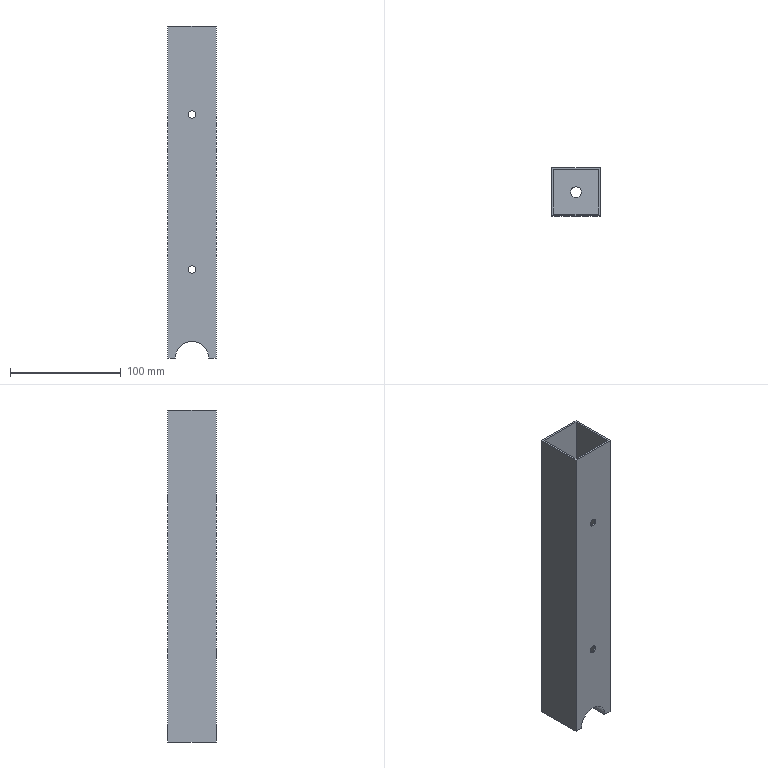Part | SolidWorks | features ICE 3, Extrusion 1, HoleWzd 1 | 1 solid | 28 faces | box 43.5 x 43.5 x 300 mm | volume 108012 mm3 | cylinder 12 | plane 12 | cone 4 | commonest cylinder face diameters 6.8 x8 10 x2 30 x2
STEP:
#1=CARTESIAN_POINT('',(-15.25,20.25,30.));
#2=VERTEX_POINT('',#1);
#3=CARTESIAN_POINT('',(-25.25,20.25,30.));
#4=VERTEX_POINT('',#3);
#5=CARTESIAN_POINT('',(-20.25,20.25,30.));
#6=DIRECTION('',(0.,0.,-1.));
#7=DIRECTION('',(-1.,0.,0.));
#8=AXIS2_PLACEMENT_3D('',#5,#6,#7);
#9=CIRCLE('',#8,5.);
#10=EDGE_CURVE('',#2,#4,#9,.T.);
#11=ORIENTED_EDGE('',*,*,#10,.F.);
#12=CARTESIAN_POINT('',(-15.25,20.25,14.142));
#13=VERTEX_POINT('',#12);
#14=CARTESIAN_POINT('',(-15.25,20.25,300.));
#15=DIRECTION('',(0.,0.,-1.));
#16=VECTOR('',#15,1000.);
#17=LINE('',#14,#16);
#18=EDGE_CURVE('',#2,#13,#17,.T.);
#19=ORIENTED_EDGE('',*,*,#18,.T.);
#20=CARTESIAN_POINT('',(-20.25,15.25,15.));
#21=VERTEX_POINT('',#20);
#22=CARTESIAN_POINT('',(-20.25,15.25,15.));
#23=CARTESIAN_POINT('',(-19.921,15.25,15.));
#24=CARTESIAN_POINT('',(-19.587,15.283,14.989));
#25=CARTESIAN_POINT('',(-18.944,15.412,14.947));
#26=CARTESIAN_POINT('',(-18.631,15.508,14.916));
#27=CARTESIAN_POINT('',(-18.023,15.761,14.837));
#28=CARTESIAN_POINT('',(-17.735,15.917,14.79));
#29=CARTESIAN_POINT('',(-17.196,16.278,14.688));
#30=CARTESIAN_POINT('',(-16.941,16.487,14.632));
#31=CARTESIAN_POINT('',(-16.481,16.948,14.521));
#32=CARTESIAN_POINT('',(-16.276,17.198,14.465));
#33=CARTESIAN_POINT('',(-15.915,17.738,14.361));
#34=CARTESIAN_POINT('',(-15.758,18.03,14.312));
#35=CARTESIAN_POINT('',(-15.508,18.632,14.231));
#36=CARTESIAN_POINT('',(-15.412,18.944,14.199));
#37=CARTESIAN_POINT('',(-15.315,19.429,14.165));
#38=CARTESIAN_POINT('',(-15.29,19.594,14.156));
#39=CARTESIAN_POINT('',(-15.258,19.922,14.145));
#40=CARTESIAN_POINT('',(-15.25,20.086,14.142));
#41=CARTESIAN_POINT('',(-15.25,20.25,14.142));
#42=B_SPLINE_CURVE_WITH_KNOTS('',3,(#22,#23,#24,#25,#26,#27,#28,#29,#30,#31,#32,#33,#34,#35,#36,#37,#38,#39,#40,#41),.UNSPECIFIED.,.F.,.F.,(4,2,2,2,2,2,2,2,2,4),(0.007875,0.008859,0.009843,0.01083,0.01181,0.01279,0.01378,0.01476,0.01525,0.01575),.UNSPECIFIED.);
#43=EDGE_CURVE('',#21,#13,#42,.T.);
#44=ORIENTED_EDGE('',*,*,#43,.F.);
#45=CARTESIAN_POINT('',(-25.25,20.25,14.142));
#46=VERTEX_POINT('',#45);
#47=CARTESIAN_POINT('',(-25.25,20.25,14.142));
#48=CARTESIAN_POINT('',(-25.25,19.917,14.142));
#49=CARTESIAN_POINT('',(-25.217,19.59,14.154));
#50=CARTESIAN_POINT('',(-25.088,18.948,14.198));
#51=CARTESIAN_POINT('',(-24.991,18.629,14.232));
#52=CARTESIAN_POINT('',(-24.739,18.024,14.313));
#53=CARTESIAN_POINT('',(-24.585,17.738,14.361));
#54=CARTESIAN_POINT('',(-24.223,17.196,14.466));
#55=CARTESIAN_POINT('',(-24.013,16.942,14.522));
#56=CARTESIAN_POINT('',(-23.555,16.484,14.633));
#57=CARTESIAN_POINT('',(-23.305,16.278,14.688));
#58=CARTESIAN_POINT('',(-22.758,15.912,14.791));
#59=CARTESIAN_POINT('',(-22.471,15.759,14.838));
#60=CARTESIAN_POINT('',(-22.02,15.571,14.896));
#61=CARTESIAN_POINT('',(-21.867,15.516,14.913));
#62=CARTESIAN_POINT('',(-21.552,15.42,14.944));
#63=CARTESIAN_POINT('',(-21.39,15.379,14.957));
#64=CARTESIAN_POINT('',(-20.905,15.282,14.989));
#65=CARTESIAN_POINT('',(-20.579,15.25,15.));
#66=CARTESIAN_POINT('',(-20.25,15.25,15.));
#67=B_SPLINE_CURVE_WITH_KNOTS('',3,(#47,#48,#49,#50,#51,#52,#53,#54,#55,#56,#57,#58,#59,#60,#61,#62,#63,#64,#65,#66),.UNSPECIFIED.,.F.,.F.,(4,2,2,2,2,2,2,2,2,4),(0.,0.0009844,0.001969,0.002953,0.003937,0.004922,0.005906,0.006398,0.006891,0.007875),.UNSPECIFIED.);
#68=EDGE_CURVE('',#46,#21,#67,.T.);
#69=ORIENTED_EDGE('',*,*,#68,.F.);
#70=CARTESIAN_POINT('',(-25.25,20.25,300.));
#71=DIRECTION('',(0.,0.,-1.));
#72=VECTOR('',#71,1000.);
#73=LINE('',#70,#72);
#74=EDGE_CURVE('',#4,#46,#73,.T.);
#75=ORIENTED_EDGE('',*,*,#74,.F.);
#76=EDGE_LOOP('',(#11,#19,#44,#69,#75));
#77=FACE_OUTER_BOUND('',#76,.T.);
#78=CARTESIAN_POINT('',(-20.25,20.25,300.));
#79=DIRECTION('',(0.,0.,-1.));
#80=DIRECTION('',(-1.,0.,0.));
#81=AXIS2_PLACEMENT_3D('',#78,#79,#80);
#82=CYLINDRICAL_SURFACE('',#81,5.);
#83=ADVANCED_FACE('',(#77),#82,.F.);
#84=CARTESIAN_POINT('',(-20.25,-1.5,15.));
#85=VERTEX_POINT('',#84);
#86=CARTESIAN_POINT('',(-5.25,-1.5,0.));
#87=VERTEX_POINT('',#86);
#88=CARTESIAN_POINT('',(-20.25,-1.5,0.));
#89=DIRECTION('',(0.,1.,0.));
#90=DIRECTION('',(0.,0.,1.));
#91=AXIS2_PLACEMENT_3D('',#88,#89,#90);
#92=CIRCLE('',#91,15.);
#93=EDGE_CURVE('',#85,#87,#92,.T.);
#94=ORIENTED_EDGE('',*,*,#93,.F.);
#95=CARTESIAN_POINT('',(-20.25,-1.5,15.));
#96=DIRECTION('',(0.,1.,0.));
#97=VECTOR('',#96,1000.);
#98=LINE('',#95,#97);
#99=EDGE_CURVE('',#85,#21,#98,.T.);
#100=ORIENTED_EDGE('',*,*,#99,.T.);
#101=ORIENTED_EDGE('',*,*,#43,.T.);
#102=CARTESIAN_POINT('',(-20.25,25.25,15.));
#103=VERTEX_POINT('',#102);
#104=CARTESIAN_POINT('',(-15.25,20.25,14.142));
#105=CARTESIAN_POINT('',(-15.25,20.578,14.142));
#106=CARTESIAN_POINT('',(-15.282,20.908,14.154));
#107=CARTESIAN_POINT('',(-15.412,21.556,14.199));
#108=CARTESIAN_POINT('',(-15.508,21.869,14.231));
#109=CARTESIAN_POINT('',(-15.759,22.472,14.313));
#110=CARTESIAN_POINT('',(-15.916,22.764,14.361));
#111=CARTESIAN_POINT('',(-16.278,23.304,14.466));
#112=CARTESIAN_POINT('',(-16.483,23.554,14.521));
#113=CARTESIAN_POINT('',(-16.945,24.016,14.633));
#114=CARTESIAN_POINT('',(-17.198,24.224,14.689));
#115=CARTESIAN_POINT('',(-17.736,24.584,14.79));
#116=CARTESIAN_POINT('',(-18.025,24.74,14.837));
#117=CARTESIAN_POINT('',(-18.633,24.993,14.916));
#118=CARTESIAN_POINT('',(-18.945,25.088,14.947));
#119=CARTESIAN_POINT('',(-19.587,25.217,14.989));
#120=CARTESIAN_POINT('',(-19.921,25.25,15.));
#121=CARTESIAN_POINT('',(-20.25,25.25,15.));
#122=B_SPLINE_CURVE_WITH_KNOTS('',3,(#104,#105,#106,#107,#108,#109,#110,#111,#112,#113,#114,#115,#116,#117,#118,#119,#120,#121),.UNSPECIFIED.,.F.,.F.,(4,2,2,2,2,2,2,2,4),(0.01575,0.01673,0.01771,0.0187,0.01968,0.02066,0.02165,0.02263,0.02362),.UNSPECIFIED.);
#123=EDGE_CURVE('',#13,#103,#122,.T.);
#124=ORIENTED_EDGE('',*,*,#123,.T.);
#125=CARTESIAN_POINT('',(-20.25,42.,15.));
#126=VERTEX_POINT('',#125);
#127=CARTESIAN_POINT('',(-20.25,-1.5,15.));
#128=DIRECTION('',(0.,1.,0.));
#129=VECTOR('',#128,1000.);
#130=LINE('',#127,#129);
#131=EDGE_CURVE('',#103,#126,#130,.T.);
#132=ORIENTED_EDGE('',*,*,#131,.T.);
#133=CARTESIAN_POINT('',(-5.25,42.,0.));
#134=VERTEX_POINT('',#133);
#135=CARTESIAN_POINT('',(-20.25,42.,0.));
#136=DIRECTION('',(0.,1.,0.));
#137=DIRECTION('',(0.,0.,1.));
#138=AXIS2_PLACEMENT_3D('',#135,#136,#137);
#139=CIRCLE('',#138,15.);
#140=EDGE_CURVE('',#126,#134,#139,.T.);
#141=ORIENTED_EDGE('',*,*,#140,.T.);
#142=CARTESIAN_POINT('',(-5.25,-1.5,0.));
#143=DIRECTION('',(0.,1.,0.));
#144=VECTOR('',#143,1000.);
#145=LINE('',#142,#144);
#146=EDGE_CURVE('',#87,#134,#145,.T.);
#147=ORIENTED_EDGE('',*,*,#146,.F.);
#148=EDGE_LOOP('',(#94,#100,#101,#124,#132,#141,#147));
#149=FACE_OUTER_BOUND('',#148,.T.);
#150=CARTESIAN_POINT('',(-20.25,-1.5,0.));
#151=DIRECTION('',(0.,1.,0.));
#152=DIRECTION('',(0.,0.,1.));
#153=AXIS2_PLACEMENT_3D('',#150,#151,#152);
#154=CYLINDRICAL_SURFACE('',#153,15.);
#155=ADVANCED_FACE('',(#149),#154,.F.);
#156=CARTESIAN_POINT('',(-20.25,-1.5,76.6));
#157=VERTEX_POINT('',#156);
#158=CARTESIAN_POINT('',(-20.25,-1.5,83.4));
#159=VERTEX_POINT('',#158);
#160=CARTESIAN_POINT('',(-20.25,-1.5,80.));
#161=DIRECTION('',(0.,1.,0.));
#162=DIRECTION('',(0.,0.,1.));
#163=AXIS2_PLACEMENT_3D('',#160,#161,#162);
#164=CIRCLE('',#163,3.4);
#165=EDGE_CURVE('',#157,#159,#164,.T.);
#166=ORIENTED_EDGE('',*,*,#165,.F.);
#167=CARTESIAN_POINT('',(-20.25,0.,76.6));
#168=VERTEX_POINT('',#167);
#169=CARTESIAN_POINT('',(-20.25,42.,76.6));
#170=DIRECTION('',(0.,1.,0.));
#171=VECTOR('',#170,1000.);
#172=LINE('',#169,#171);
#173=EDGE_CURVE('',#157,#168,#172,.T.);
#174=ORIENTED_EDGE('',*,*,#173,.T.);
#175=CARTESIAN_POINT('',(-20.25,0.,83.4));
#176=VERTEX_POINT('',#175);
#177=CARTESIAN_POINT('',(-20.25,0.,80.));
#178=DIRECTION('',(0.,1.,0.));
#179=DIRECTION('',(0.,0.,1.));
#180=AXIS2_PLACEMENT_3D('',#177,#178,#179);
#181=CIRCLE('',#180,3.4);
#182=EDGE_CURVE('',#168,#176,#181,.T.);
#183=ORIENTED_EDGE('',*,*,#182,.T.);
#184=CARTESIAN_POINT('',(-20.25,42.,83.4));
#185=DIRECTION('',(0.,1.,0.));
#186=VECTOR('',#185,1000.);
#187=LINE('',#184,#186);
#188=EDGE_CURVE('',#159,#176,#187,.T.);
#189=ORIENTED_EDGE('',*,*,#188,.F.);
#190=EDGE_LOOP('',(#166,#174,#183,#189));
#191=FACE_OUTER_BOUND('',#190,.T.);
#192=CARTESIAN_POINT('',(-20.25,42.,80.));
#193=DIRECTION('',(0.,1.,0.));
#194=DIRECTION('',(0.,0.,1.));
#195=AXIS2_PLACEMENT_3D('',#192,#193,#194);
#196=CYLINDRICAL_SURFACE('',#195,3.4);
#197=ADVANCED_FACE('',(#191),#196,.F.);
#198=CARTESIAN_POINT('',(-20.25,40.5,83.4));
#199=VERTEX_POINT('',#198);
#200=CARTESIAN_POINT('',(-20.25,40.5,76.6));
#201=VERTEX_POINT('',#200);
#202=CARTESIAN_POINT('',(-20.25,40.5,80.));
#203=DIRECTION('',(0.,-1.,0.));
#204=DIRECTION('',(1.,0.,0.));
#205=AXIS2_PLACEMENT_3D('',#202,#203,#204);
#206=CIRCLE('',#205,3.4);
#207=EDGE_CURVE('',#199,#201,#206,.T.);
#208=ORIENTED_EDGE('',*,*,#207,.T.);
#209=CARTESIAN_POINT('',(-20.25,41.375,76.6));
#210=VERTEX_POINT('',#209);
#211=CARTESIAN_POINT('',(-20.25,42.,76.6));
#212=DIRECTION('',(0.,1.,0.));
#213=VECTOR('',#212,1000.);
#214=LINE('',#211,#213);
#215=EDGE_CURVE('',#201,#210,#214,.T.);
#216=ORIENTED_EDGE('',*,*,#215,.T.);
#217=CARTESIAN_POINT('',(-20.25,41.375,83.4));
#218=VERTEX_POINT('',#217);
#219=CARTESIAN_POINT('',(-20.25,41.375,80.));
#220=DIRECTION('',(0.,1.,0.));
#221=DIRECTION('',(0.,0.,1.));
#222=AXIS2_PLACEMENT_3D('',#219,#220,#221);
#223=CIRCLE('',#222,3.4);
#224=EDGE_CURVE('',#210,#218,#223,.T.);
#225=ORIENTED_EDGE('',*,*,#224,.T.);
#226=CARTESIAN_POINT('',(-20.25,42.,83.4));
#227=DIRECTION('',(0.,1.,0.));
#228=VECTOR('',#227,1000.);
#229=LINE('',#226,#228);
#230=EDGE_CURVE('',#199,#218,#229,.T.);
#231=ORIENTED_EDGE('',*,*,#230,.F.);
#232=EDGE_LOOP('',(#208,#216,#225,#231));
#233=FACE_OUTER_BOUND('',#232,.T.);
#234=CARTESIAN_POINT('',(-20.25,42.,80.));
#235=DIRECTION('',(0.,1.,0.));
#236=DIRECTION('',(0.,0.,1.));
#237=AXIS2_PLACEMENT_3D('',#234,#235,#236);
#238=CYLINDRICAL_SURFACE('',#237,3.4);
#239=ADVANCED_FACE('',(#233),#238,.F.);
#240=ORIENTED_EDGE('',*,*,#224,.F.);
#241=CARTESIAN_POINT('',(-20.25,42.,75.975));
#242=VERTEX_POINT('',#241);
#243=CARTESIAN_POINT('',(-20.25,42.,75.975));
#244=DIRECTION('',(0.,0.7071,-0.7071));
#245=VECTOR('',#244,1000.);
#246=LINE('',#243,#245);
#247=EDGE_CURVE('',#210,#242,#246,.T.);
#248=ORIENTED_EDGE('',*,*,#247,.T.);
#249=CARTESIAN_POINT('',(-20.25,42.,84.025));
#250=VERTEX_POINT('',#249);
#251=CARTESIAN_POINT('',(-20.25,42.,80.));
#252=DIRECTION('',(0.,1.,0.));
#253=DIRECTION('',(0.,0.,1.));
#254=AXIS2_PLACEMENT_3D('',#251,#252,#253);
#255=CIRCLE('',#254,4.025);
#256=EDGE_CURVE('',#242,#250,#255,.T.);
#257=ORIENTED_EDGE('',*,*,#256,.T.);
#258=CARTESIAN_POINT('',(-20.25,42.,84.025));
#259=DIRECTION('',(0.,0.7071,0.7071));
#260=VECTOR('',#259,1000.);
#261=LINE('',#258,#260);
#262=EDGE_CURVE('',#218,#250,#261,.T.);
#263=ORIENTED_EDGE('',*,*,#262,.F.);
#264=EDGE_LOOP('',(#240,#248,#257,#263));
#265=FACE_OUTER_BOUND('',#264,.T.);
#266=CARTESIAN_POINT('',(-20.25,42.,80.));
#267=DIRECTION('',(0.,1.,0.));
#268=DIRECTION('',(0.,0.,1.));
#269=AXIS2_PLACEMENT_3D('',#266,#267,#268);
#270=CONICAL_SURFACE('',#269,4.025,0.7854);
#271=ADVANCED_FACE('',(#265),#270,.F.);
#272=CARTESIAN_POINT('',(-20.25,41.375,216.6));
#273=VERTEX_POINT('',#272);
#274=CARTESIAN_POINT('',(-20.25,41.375,223.4));
#275=VERTEX_POINT('',#274);
#276=CARTESIAN_POINT('',(-20.25,41.375,220.));
#277=DIRECTION('',(0.,1.,0.));
#278=DIRECTION('',(0.,0.,1.));
#279=AXIS2_PLACEMENT_3D('',#276,#277,#278);
#280=CIRCLE('',#279,3.4);
#281=EDGE_CURVE('',#273,#275,#280,.T.);
#282=ORIENTED_EDGE('',*,*,#281,.F.);
#283=CARTESIAN_POINT('',(-20.25,42.,215.975));
#284=VERTEX_POINT('',#283);
#285=CARTESIAN_POINT('',(-20.25,42.,215.975));
#286=DIRECTION('',(0.,0.7071,-0.7071));
#287=VECTOR('',#286,1000.);
#288=LINE('',#285,#287);
#289=EDGE_CURVE('',#273,#284,#288,.T.);
#290=ORIENTED_EDGE('',*,*,#289,.T.);
#291=CARTESIAN_POINT('',(-20.25,42.,224.025));
#292=VERTEX_POINT('',#291);
#293=CARTESIAN_POINT('',(-20.25,42.,220.));
#294=DIRECTION('',(0.,1.,0.));
#295=DIRECTION('',(0.,0.,1.));
#296=AXIS2_PLACEMENT_3D('',#293,#294,#295);
#297=CIRCLE('',#296,4.025);
#298=EDGE_CURVE('',#284,#292,#297,.T.);
#299=ORIENTED_EDGE('',*,*,#298,.T.);
#300=CARTESIAN_POINT('',(-20.25,42.,224.025));
#301=DIRECTION('',(0.,0.7071,0.7071));
#302=VECTOR('',#301,1000.);
#303=LINE('',#300,#302);
#304=EDGE_CURVE('',#275,#292,#303,.T.);
#305=ORIENTED_EDGE('',*,*,#304,.F.);
#306=EDGE_LOOP('',(#282,#290,#299,#305));
#307=FACE_OUTER_BOUND('',#306,.T.);
#308=CARTESIAN_POINT('',(-20.25,42.,220.));
#309=DIRECTION('',(0.,1.,0.));
#310=DIRECTION('',(0.,0.,1.));
#311=AXIS2_PLACEMENT_3D('',#308,#309,#310);
#312=CONICAL_SURFACE('',#311,4.025,0.7854);
#313=ADVANCED_FACE('',(#307),#312,.F.);
#314=CARTESIAN_POINT('',(-20.25,40.5,223.4));
#315=VERTEX_POINT('',#314);
#316=CARTESIAN_POINT('',(-20.25,40.5,216.6));
#317=VERTEX_POINT('',#316);
#318=CARTESIAN_POINT('',(-20.25,40.5,220.));
#319=DIRECTION('',(0.,-1.,0.));
#320=DIRECTION('',(1.,0.,0.));
#321=AXIS2_PLACEMENT_3D('',#318,#319,#320);
#322=CIRCLE('',#321,3.4);
#323=EDGE_CURVE('',#315,#317,#322,.T.);
#324=ORIENTED_EDGE('',*,*,#323,.T.);
#325=CARTESIAN_POINT('',(-20.25,42.,216.6));
#326=DIRECTION('',(0.,1.,0.));
#327=VECTOR('',#326,1000.);
#328=LINE('',#325,#327);
#329=EDGE_CURVE('',#317,#273,#328,.T.);
#330=ORIENTED_EDGE('',*,*,#329,.T.);
#331=ORIENTED_EDGE('',*,*,#281,.T.);
#332=CARTESIAN_POINT('',(-20.25,42.,223.4));
#333=DIRECTION('',(0.,1.,0.));
#334=VECTOR('',#333,1000.);
#335=LINE('',#332,#334);
#336=EDGE_CURVE('',#315,#275,#335,.T.);
#337=ORIENTED_EDGE('',*,*,#336,.F.);
#338=EDGE_LOOP('',(#324,#330,#331,#337));
#339=FACE_OUTER_BOUND('',#338,.T.);
#340=CARTESIAN_POINT('',(-20.25,42.,220.));
#341=DIRECTION('',(0.,1.,0.));
#342=DIRECTION('',(0.,0.,1.));
#343=AXIS2_PLACEMENT_3D('',#340,#341,#342);
#344=CYLINDRICAL_SURFACE('',#343,3.4);
#345=ADVANCED_FACE('',(#339),#344,.F.);
#346=CARTESIAN_POINT('',(-20.25,-1.5,216.6));
#347=VERTEX_POINT('',#346);
#348=CARTESIAN_POINT('',(-20.25,-1.5,223.4));
#349=VERTEX_POINT('',#348);
#350=CARTESIAN_POINT('',(-20.25,-1.5,220.));
#351=DIRECTION('',(0.,1.,0.));
#352=DIRECTION('',(0.,0.,1.));
#353=AXIS2_PLACEMENT_3D('',#350,#351,#352);
#354=CIRCLE('',#353,3.4);
#355=EDGE_CURVE('',#347,#349,#354,.T.);
#356=ORIENTED_EDGE('',*,*,#355,.F.);
#357=CARTESIAN_POINT('',(-20.25,0.,216.6));
#358=VERTEX_POINT('',#357);
#359=CARTESIAN_POINT('',(-20.25,42.,216.6));
#360=DIRECTION('',(0.,1.,0.));
#361=VECTOR('',#360,1000.);
#362=LINE('',#359,#361);
#363=EDGE_CURVE('',#347,#358,#362,.T.);
#364=ORIENTED_EDGE('',*,*,#363,.T.);
#365=CARTESIAN_POINT('',(-20.25,0.,223.4));
#366=VERTEX_POINT('',#365);
#367=CARTESIAN_POINT('',(-20.25,0.,220.));
#368=DIRECTION('',(0.,1.,0.));
#369=DIRECTION('',(0.,0.,1.));
#370=AXIS2_PLACEMENT_3D('',#367,#368,#369);
#371=CIRCLE('',#370,3.4);
#372=EDGE_CURVE('',#358,#366,#371,.T.);
#373=ORIENTED_EDGE('',*,*,#372,.T.);
#374=CARTESIAN_POINT('',(-20.25,42.,223.4));
#375=DIRECTION('',(0.,1.,0.));
#376=VECTOR('',#375,1000.);
#377=LINE('',#374,#376);
#378=EDGE_CURVE('',#349,#366,#377,.T.);
#379=ORIENTED_EDGE('',*,*,#378,.F.);
#380=EDGE_LOOP('',(#356,#364,#373,#379));
#381=FACE_OUTER_BOUND('',#380,.T.);
#382=CARTESIAN_POINT('',(-20.25,42.,220.));
#383=DIRECTION('',(0.,1.,0.));
#384=DIRECTION('',(0.,0.,1.));
#385=AXIS2_PLACEMENT_3D('',#382,#383,#384);
#386=CYLINDRICAL_SURFACE('',#385,3.4);
#387=ADVANCED_FACE('',(#381),#386,.F.);
#388=CARTESIAN_POINT('',(1.5,-1.5,0.));
#389=VERTEX_POINT('',#388);
#390=CARTESIAN_POINT('',(-42.,-1.5,0.));
#391=DIRECTION('',(1.,0.,0.));
#392=VECTOR('',#391,1000.);
#393=LINE('',#390,#392);
#394=EDGE_CURVE('',#87,#389,#393,.T.);
#395=ORIENTED_EDGE('',*,*,#394,.F.);
#396=ORIENTED_EDGE('',*,*,#146,.T.);
#397=CARTESIAN_POINT('',(1.5,42.,0.));
#398=VERTEX_POINT('',#397);
#399=CARTESIAN_POINT('',(-42.,42.,0.));
#400=DIRECTION('',(-1.,0.,0.));
#401=VECTOR('',#400,1000.);
#402=LINE('',#399,#401);
#403=EDGE_CURVE('',#398,#134,#402,.T.);
#404=ORIENTED_EDGE('',*,*,#403,.F.);
#405=CARTESIAN_POINT('',(1.5,42.,0.));
#406=DIRECTION('',(0.,1.,0.));
#407=VECTOR('',#406,1000.);
#408=LINE('',#405,#407);
#409=EDGE_CURVE('',#389,#398,#408,.T.);
#410=ORIENTED_EDGE('',*,*,#409,.F.);
#411=EDGE_LOOP('',(#395,#396,#404,#410));
#412=FACE_OUTER_BOUND('',#411,.T.);
#413=CARTESIAN_POINT('',(0.,0.,0.));
#414=DIRECTION('',(0.,0.,1.));
#415=DIRECTION('',(1.,0.,0.));
#416=AXIS2_PLACEMENT_3D('',#413,#414,#415);
#417=PLANE('',#416);
#418=ADVANCED_FACE('',(#412),#417,.F.);
#419=CARTESIAN_POINT('',(-40.5,0.,300.));
#420=VERTEX_POINT('',#419);
#421=CARTESIAN_POINT('',(-40.5,0.,30.));
#422=VERTEX_POINT('',#421);
#423=CARTESIAN_POINT('',(-40.5,0.,300.));
#424=DIRECTION('',(0.,0.,-1.));
#425=VECTOR('',#424,1000.);
#426=LINE('',#423,#425);
#427=EDGE_CURVE('',#420,#422,#426,.T.);
#428=ORIENTED_EDGE('',*,*,#427,.T.);
#429=CARTESIAN_POINT('',(-40.5,40.5,30.));
#430=VERTEX_POINT('',#429);
#431=CARTESIAN_POINT('',(-40.5,40.5,30.));
#432=DIRECTION('',(0.,1.,0.));
#433=VECTOR('',#432,1000.);
#434=LINE('',#431,#433);
#435=EDGE_CURVE('',#422,#430,#434,.T.);
#436=ORIENTED_EDGE('',*,*,#435,.T.);
#437=CARTESIAN_POINT('',(-40.5,40.5,300.));
#438=VERTEX_POINT('',#437);
#439=CARTESIAN_POINT('',(-40.5,40.5,300.));
#440=DIRECTION('',(0.,0.,-1.));
#441=VECTOR('',#440,1000.);
#442=LINE('',#439,#441);
#443=EDGE_CURVE('',#438,#430,#442,.T.);
#444=ORIENTED_EDGE('',*,*,#443,.F.);
#445=CARTESIAN_POINT('',(-40.5,40.5,300.));
#446=DIRECTION('',(0.,-1.,0.));
#447=VECTOR('',#446,1000.);
#448=LINE('',#445,#447);
#449=EDGE_CURVE('',#438,#420,#448,.T.);
#450=ORIENTED_EDGE('',*,*,#449,.T.);
#451=EDGE_LOOP('',(#428,#436,#444,#450));
#452=FACE_OUTER_BOUND('',#451,.T.);
#453=CARTESIAN_POINT('',(-40.5,40.5,300.));
#454=DIRECTION('',(1.,0.,0.));
#455=DIRECTION('',(0.,1.,0.));
#456=AXIS2_PLACEMENT_3D('',#453,#454,#455);
#457=PLANE('',#456);
#458=ADVANCED_FACE('',(#452),#457,.T.);
#459=CARTESIAN_POINT('',(-20.25,0.,80.));
#460=DIRECTION('',(0.,1.,0.));
#461=DIRECTION('',(0.,0.,1.));
#462=AXIS2_PLACEMENT_3D('',#459,#460,#461);
#463=CIRCLE('',#462,3.4);
#464=EDGE_CURVE('',#176,#168,#463,.T.);
#465=ORIENTED_EDGE('',*,*,#464,.F.);
#466=ORIENTED_EDGE('',*,*,#182,.F.);
#467=EDGE_LOOP('',(#465,#466));
#468=FACE_BOUND('',#467,.T.);
#469=CARTESIAN_POINT('',(-20.25,0.,220.));
#470=DIRECTION('',(0.,1.,0.));
#471=DIRECTION('',(0.,0.,1.));
#472=AXIS2_PLACEMENT_3D('',#469,#470,#471);
#473=CIRCLE('',#472,3.4);
#474=EDGE_CURVE('',#366,#358,#473,.T.);
#475=ORIENTED_EDGE('',*,*,#474,.F.);
#476=ORIENTED_EDGE('',*,*,#372,.F.);
#477=EDGE_LOOP('',(#475,#476));
#478=FACE_BOUND('',#477,.T.);
#479=CARTESIAN_POINT('',(0.,0.,300.));
#480=VERTEX_POINT('',#479);
#481=CARTESIAN_POINT('',(0.,0.,30.));
#482=VERTEX_POINT('',#481);
#483=CARTESIAN_POINT('',(0.,0.,300.));
#484=DIRECTION('',(0.,0.,-1.));
#485=VECTOR('',#484,1000.);
#486=LINE('',#483,#485);
#487=EDGE_CURVE('',#480,#482,#486,.T.);
#488=ORIENTED_EDGE('',*,*,#487,.T.);
#489=CARTESIAN_POINT('',(-40.5,0.,30.));
#490=DIRECTION('',(-1.,0.,0.));
#491=VECTOR('',#490,1000.);
#492=LINE('',#489,#491);
#493=EDGE_CURVE('',#482,#422,#492,.T.);
#494=ORIENTED_EDGE('',*,*,#493,.T.);
#495=ORIENTED_EDGE('',*,*,#427,.F.);
#496=CARTESIAN_POINT('',(-40.5,0.,300.));
#497=DIRECTION('',(1.,0.,0.));
#498=VECTOR('',#497,1000.);
#499=LINE('',#496,#498);
#500=EDGE_CURVE('',#420,#480,#499,.T.);
#501=ORIENTED_EDGE('',*,*,#500,.T.);
#502=EDGE_LOOP('',(#488,#494,#495,#501));
#503=FACE_OUTER_BOUND('',#502,.T.);
#504=CARTESIAN_POINT('',(-40.5,0.,300.));
#505=DIRECTION('',(0.,1.,0.));
#506=DIRECTION('',(0.,0.,1.));
#507=AXIS2_PLACEMENT_3D('',#504,#505,#506);
#508=PLANE('',#507);
#509=ADVANCED_FACE('',(#468,#478,#503),#508,.T.);
#510=CARTESIAN_POINT('',(0.,40.5,300.));
#511=VERTEX_POINT('',#510);
#512=CARTESIAN_POINT('',(0.,40.5,30.));
#513=VERTEX_POINT('',#512);
#514=CARTESIAN_POINT('',(0.,40.5,300.));
#515=DIRECTION('',(0.,0.,-1.));
#516=VECTOR('',#515,1000.);
#517=LINE('',#514,#516);
#518=EDGE_CURVE('',#511,#513,#517,.T.);
#519=ORIENTED_EDGE('',*,*,#518,.T.);
#520=CARTESIAN_POINT('',(0.,40.5,30.));
#521=DIRECTION('',(0.,-1.,0.));
#522=VECTOR('',#521,1000.);
#523=LINE('',#520,#522);
#524=EDGE_CURVE('',#513,#482,#523,.T.);
#525=ORIENTED_EDGE('',*,*,#524,.T.);
#526=ORIENTED_EDGE('',*,*,#487,.F.);
#527=CARTESIAN_POINT('',(0.,40.5,300.));
#528=DIRECTION('',(0.,1.,0.));
#529=VECTOR('',#528,1000.);
#530=LINE('',#527,#529);
#531=EDGE_CURVE('',#480,#511,#530,.T.);
#532=ORIENTED_EDGE('',*,*,#531,.T.);
#533=EDGE_LOOP('',(#519,#525,#526,#532));
#534=FACE_OUTER_BOUND('',#533,.T.);
#535=CARTESIAN_POINT('',(0.,40.5,300.));
#536=DIRECTION('',(-1.,0.,0.));
#537=DIRECTION('',(0.,-1.,0.));
#538=AXIS2_PLACEMENT_3D('',#535,#536,#537);
#539=PLANE('',#538);
#540=ADVANCED_FACE('',(#534),#539,.T.);
#541=ORIENTED_EDGE('',*,*,#207,.F.);
#542=CARTESIAN_POINT('',(-20.25,40.5,80.));
#543=DIRECTION('',(0.,-1.,0.));
#544=DIRECTION('',(1.,0.,0.));
#545=AXIS2_PLACEMENT_3D('',#542,#543,#544);
#546=CIRCLE('',#545,3.4);
#547=EDGE_CURVE('',#201,#199,#546,.T.);
#548=ORIENTED_EDGE('',*,*,#547,.F.);
#549=EDGE_LOOP('',(#541,#548));
#550=FACE_BOUND('',#549,.T.);
#551=ORIENTED_EDGE('',*,*,#323,.F.);
#552=CARTESIAN_POINT('',(-20.25,40.5,220.));
#553=DIRECTION('',(0.,-1.,0.));
#554=DIRECTION('',(1.,0.,0.));
#555=AXIS2_PLACEMENT_3D('',#552,#553,#554);
#556=CIRCLE('',#555,3.4);
#557=EDGE_CURVE('',#317,#315,#556,.T.);
#558=ORIENTED_EDGE('',*,*,#557,.F.);
#559=EDGE_LOOP('',(#551,#558));
#560=FACE_BOUND('',#559,.T.);
#561=ORIENTED_EDGE('',*,*,#443,.T.);
#562=CARTESIAN_POINT('',(-40.5,40.5,30.));
#563=DIRECTION('',(1.,0.,0.));
#564=VECTOR('',#563,1000.);
#565=LINE('',#562,#564);
#566=EDGE_CURVE('',#430,#513,#565,.T.);
#567=ORIENTED_EDGE('',*,*,#566,.T.);
#568=ORIENTED_EDGE('',*,*,#518,.F.);
#569=CARTESIAN_POINT('',(-40.5,40.5,300.));
#570=DIRECTION('',(-1.,0.,0.));
#571=VECTOR('',#570,1000.);
#572=LINE('',#569,#571);
#573=EDGE_CURVE('',#511,#438,#572,.T.);
#574=ORIENTED_EDGE('',*,*,#573,.T.);
#575=EDGE_LOOP('',(#561,#567,#568,#574));
#576=FACE_OUTER_BOUND('',#575,.T.);
#577=CARTESIAN_POINT('',(-40.5,40.5,300.));
#578=DIRECTION('',(0.,-1.,0.));
#579=DIRECTION('',(1.,0.,0.));
#580=AXIS2_PLACEMENT_3D('',#577,#578,#579);
#581=PLANE('',#580);
#582=ADVANCED_FACE('',(#550,#560,#576),#581,.T.);
#583=CARTESIAN_POINT('',(-42.,42.,300.));
#584=VERTEX_POINT('',#583);
#585=CARTESIAN_POINT('',(-42.,-1.5,300.));
#586=VERTEX_POINT('',#585);
#587=CARTESIAN_POINT('',(-42.,42.,300.));
#588=DIRECTION('',(0.,-1.,0.));
#589=VECTOR('',#588,1000.);
#590=LINE('',#587,#589);
#591=EDGE_CURVE('',#584,#586,#590,.T.);
#592=ORIENTED_EDGE('',*,*,#591,.T.);
#593=CARTESIAN_POINT('',(1.5,-1.5,300.));
#594=VERTEX_POINT('',#593);
#595=CARTESIAN_POINT('',(-42.,-1.5,300.));
#596=DIRECTION('',(1.,0.,0.));
#597=VECTOR('',#596,1000.);
#598=LINE('',#595,#597);
#599=EDGE_CURVE('',#586,#594,#598,.T.);
#600=ORIENTED_EDGE('',*,*,#599,.T.);
#601=CARTESIAN_POINT('',(1.5,42.,300.));
#602=VERTEX_POINT('',#601);
#603=CARTESIAN_POINT('',(1.5,42.,300.));
#604=DIRECTION('',(0.,1.,0.));
#605=VECTOR('',#604,1000.);
#606=LINE('',#603,#605);
#607=EDGE_CURVE('',#594,#602,#606,.T.);
#608=ORIENTED_EDGE('',*,*,#607,.T.);
#609=CARTESIAN_POINT('',(-42.,42.,300.));
#610=DIRECTION('',(-1.,0.,0.));
#611=VECTOR('',#610,1000.);
#612=LINE('',#609,#611);
#613=EDGE_CURVE('',#602,#584,#612,.T.);
#614=ORIENTED_EDGE('',*,*,#613,.T.);
#615=EDGE_LOOP('',(#592,#600,#608,#614));
#616=FACE_OUTER_BOUND('',#615,.T.);
#617=ORIENTED_EDGE('',*,*,#500,.F.);
#618=ORIENTED_EDGE('',*,*,#449,.F.);
#619=ORIENTED_EDGE('',*,*,#573,.F.);
#620=ORIENTED_EDGE('',*,*,#531,.F.);
#621=EDGE_LOOP('',(#617,#618,#619,#620));
#622=FACE_BOUND('',#621,.T.);
#623=CARTESIAN_POINT('',(0.,0.,300.));
#624=DIRECTION('',(0.,0.,1.));
#625=DIRECTION('',(1.,0.,0.));
#626=AXIS2_PLACEMENT_3D('',#623,#624,#625);
#627=PLANE('',#626);
#628=ADVANCED_FACE('',(#616,#622),#627,.T.);
#629=CARTESIAN_POINT('',(-35.25,42.,0.));
#630=VERTEX_POINT('',#629);
#631=CARTESIAN_POINT('',(-42.,42.,0.));
#632=VERTEX_POINT('',#631);
#633=CARTESIAN_POINT('',(-42.,42.,0.));
#634=DIRECTION('',(-1.,0.,0.));
#635=VECTOR('',#634,1000.);
#636=LINE('',#633,#635);
#637=EDGE_CURVE('',#630,#632,#636,.T.);
#638=ORIENTED_EDGE('',*,*,#637,.F.);
#639=CARTESIAN_POINT('',(-35.25,-1.5,0.));
#640=VERTEX_POINT('',#639);
#641=CARTESIAN_POINT('',(-35.25,-1.5,0.));
#642=DIRECTION('',(0.,1.,0.));
#643=VECTOR('',#642,1000.);
#644=LINE('',#641,#643);
#645=EDGE_CURVE('',#640,#630,#644,.T.);
#646=ORIENTED_EDGE('',*,*,#645,.F.);
#647=CARTESIAN_POINT('',(-42.,-1.5,0.));
#648=VERTEX_POINT('',#647);
#649=CARTESIAN_POINT('',(-42.,-1.5,0.));
#650=DIRECTION('',(1.,0.,0.));
#651=VECTOR('',#650,1000.);
#652=LINE('',#649,#651);
#653=EDGE_CURVE('',#648,#640,#652,.T.);
#654=ORIENTED_EDGE('',*,*,#653,.F.);
#655=CARTESIAN_POINT('',(-42.,42.,0.));
#656=DIRECTION('',(0.,-1.,0.));
#657=VECTOR('',#656,1000.);
#658=LINE('',#655,#657);
#659=EDGE_CURVE('',#632,#648,#658,.T.);
#660=ORIENTED_EDGE('',*,*,#659,.F.);
#661=EDGE_LOOP('',(#638,#646,#654,#660));
#662=FACE_OUTER_BOUND('',#661,.T.);
#663=CARTESIAN_POINT('',(0.,0.,0.));
#664=DIRECTION('',(0.,0.,1.));
#665=DIRECTION('',(1.,0.,0.));
#666=AXIS2_PLACEMENT_3D('',#663,#664,#665);
#667=PLANE('',#666);
#668=ADVANCED_FACE('',(#662),#667,.F.);
#669=ORIENTED_EDGE('',*,*,#659,.T.);
#670=CARTESIAN_POINT('',(-42.,-1.5,300.));
#671=DIRECTION('',(0.,0.,-1.));
#672=VECTOR('',#671,1000.);
#673=LINE('',#670,#672);
#674=EDGE_CURVE('',#586,#648,#673,.T.);
#675=ORIENTED_EDGE('',*,*,#674,.F.);
#676=ORIENTED_EDGE('',*,*,#591,.F.);
#677=CARTESIAN_POINT('',(-42.,42.,300.));
#678=DIRECTION('',(0.,0.,-1.));
#679=VECTOR('',#678,1000.);
#680=LINE('',#677,#679);
#681=EDGE_CURVE('',#584,#632,#680,.T.);
#682=ORIENTED_EDGE('',*,*,#681,.T.);
#683=EDGE_LOOP('',(#669,#675,#676,#682));
#684=FACE_OUTER_BOUND('',#683,.T.);
#685=CARTESIAN_POINT('',(-42.,42.,300.));
#686=DIRECTION('',(1.,0.,0.));
#687=DIRECTION('',(0.,1.,0.));
#688=AXIS2_PLACEMENT_3D('',#685,#686,#687);
#689=PLANE('',#688);
#690=ADVANCED_FACE('',(#684),#689,.F.);
#691=CARTESIAN_POINT('',(-20.25,-1.5,80.));
#692=DIRECTION('',(0.,1.,0.));
#693=DIRECTION('',(0.,0.,1.));
#694=AXIS2_PLACEMENT_3D('',#691,#692,#693);
#695=CIRCLE('',#694,3.4);
#696=EDGE_CURVE('',#159,#157,#695,.T.);
#697=ORIENTED_EDGE('',*,*,#696,.T.);
#698=ORIENTED_EDGE('',*,*,#165,.T.);
#699=EDGE_LOOP('',(#697,#698));
#700=FACE_BOUND('',#699,.T.);
#701=CARTESIAN_POINT('',(-20.25,-1.5,220.));
#702=DIRECTION('',(0.,1.,0.));
#703=DIRECTION('',(0.,0.,1.));
#704=AXIS2_PLACEMENT_3D('',#701,#702,#703);
#705=CIRCLE('',#704,3.4);
#706=EDGE_CURVE('',#349,#347,#705,.T.);
#707=ORIENTED_EDGE('',*,*,#706,.T.);
#708=ORIENTED_EDGE('',*,*,#355,.T.);
#709=EDGE_LOOP('',(#707,#708));
#710=FACE_BOUND('',#709,.T.);
#711=ORIENTED_EDGE('',*,*,#653,.T.);
#712=CARTESIAN_POINT('',(-20.25,-1.5,0.));
#713=DIRECTION('',(0.,1.,0.));
#714=DIRECTION('',(0.,0.,1.));
#715=AXIS2_PLACEMENT_3D('',#712,#713,#714);
#716=CIRCLE('',#715,15.);
#717=EDGE_CURVE('',#640,#85,#716,.T.);
#718=ORIENTED_EDGE('',*,*,#717,.T.);
#719=ORIENTED_EDGE('',*,*,#93,.T.);
#720=ORIENTED_EDGE('',*,*,#394,.T.);
#721=CARTESIAN_POINT('',(1.5,-1.5,300.));
#722=DIRECTION('',(0.,0.,-1.));
#723=VECTOR('',#722,1000.);
#724=LINE('',#721,#723);
#725=EDGE_CURVE('',#594,#389,#724,.T.);
#726=ORIENTED_EDGE('',*,*,#725,.F.);
#727=ORIENTED_EDGE('',*,*,#599,.F.);
#728=ORIENTED_EDGE('',*,*,#674,.T.);
#729=EDGE_LOOP('',(#711,#718,#719,#720,#726,#727,#728));
#730=FACE_OUTER_BOUND('',#729,.T.);
#731=CARTESIAN_POINT('',(-42.,-1.5,300.));
#732=DIRECTION('',(0.,1.,0.));
#733=DIRECTION('',(-1.,0.,0.));
#734=AXIS2_PLACEMENT_3D('',#731,#732,#733);
#735=PLANE('',#734);
#736=ADVANCED_FACE('',(#700,#710,#730),#735,.F.);
#737=ORIENTED_EDGE('',*,*,#409,.T.);
#738=CARTESIAN_POINT('',(1.5,42.,300.));
#739=DIRECTION('',(0.,0.,-1.));
#740=VECTOR('',#739,1000.);
#741=LINE('',#738,#740);
#742=EDGE_CURVE('',#602,#398,#741,.T.);
#743=ORIENTED_EDGE('',*,*,#742,.F.);
#744=ORIENTED_EDGE('',*,*,#607,.F.);
#745=ORIENTED_EDGE('',*,*,#725,.T.);
#746=EDGE_LOOP('',(#737,#743,#744,#745));
#747=FACE_OUTER_BOUND('',#746,.T.);
#748=CARTESIAN_POINT('',(1.5,42.,300.));
#749=DIRECTION('',(-1.,0.,0.));
#750=DIRECTION('',(0.,-1.,0.));
#751=AXIS2_PLACEMENT_3D('',#748,#749,#750);
#752=PLANE('',#751);
#753=ADVANCED_FACE('',(#747),#752,.F.);
#754=CARTESIAN_POINT('',(-20.25,42.,80.));
#755=DIRECTION('',(0.,1.,0.));
#756=DIRECTION('',(0.,0.,1.));
#757=AXIS2_PLACEMENT_3D('',#754,#755,#756);
#758=CIRCLE('',#757,4.025);
#759=EDGE_CURVE('',#250,#242,#758,.T.);
#760=ORIENTED_EDGE('',*,*,#759,.F.);
#761=ORIENTED_EDGE('',*,*,#256,.F.);
#762=EDGE_LOOP('',(#760,#761));
#763=FACE_BOUND('',#762,.T.);
#764=CARTESIAN_POINT('',(-20.25,42.,220.));
#765=DIRECTION('',(0.,1.,0.));
#766=DIRECTION('',(0.,0.,1.));
#767=AXIS2_PLACEMENT_3D('',#764,#765,#766);
#768=CIRCLE('',#767,4.025);
#769=EDGE_CURVE('',#292,#284,#768,.T.);
#770=ORIENTED_EDGE('',*,*,#769,.F.);
#771=ORIENTED_EDGE('',*,*,#298,.F.);
#772=EDGE_LOOP('',(#770,#771));
#773=FACE_BOUND('',#772,.T.);
#774=ORIENTED_EDGE('',*,*,#403,.T.);
#775=ORIENTED_EDGE('',*,*,#140,.F.);
#776=CARTESIAN_POINT('',(-20.25,42.,0.));
#777=DIRECTION('',(0.,1.,0.));
#778=DIRECTION('',(0.,0.,1.));
#779=AXIS2_PLACEMENT_3D('',#776,#777,#778);
#780=CIRCLE('',#779,15.);
#781=EDGE_CURVE('',#630,#126,#780,.T.);
#782=ORIENTED_EDGE('',*,*,#781,.F.);
#783=ORIENTED_EDGE('',*,*,#637,.T.);
#784=ORIENTED_EDGE('',*,*,#681,.F.);
#785=ORIENTED_EDGE('',*,*,#613,.F.);
#786=ORIENTED_EDGE('',*,*,#742,.T.);
#787=EDGE_LOOP('',(#774,#775,#782,#783,#784,#785,#786));
#788=FACE_OUTER_BOUND('',#787,.T.);
#789=CARTESIAN_POINT('',(-42.,42.,300.));
#790=DIRECTION('',(0.,-1.,0.));
#791=DIRECTION('',(0.,0.,-1.));
#792=AXIS2_PLACEMENT_3D('',#789,#790,#791);
#793=PLANE('',#792);
#794=ADVANCED_FACE('',(#763,#773,#788),#793,.F.);
#795=CARTESIAN_POINT('',(-20.25,20.25,30.));
#796=DIRECTION('',(0.,0.,-1.));
#797=DIRECTION('',(-1.,0.,0.));
#798=AXIS2_PLACEMENT_3D('',#795,#796,#797);
#799=CIRCLE('',#798,5.);
#800=EDGE_CURVE('',#4,#2,#799,.T.);
#801=ORIENTED_EDGE('',*,*,#800,.T.);
#802=ORIENTED_EDGE('',*,*,#10,.T.);
#803=EDGE_LOOP('',(#801,#802));
#804=FACE_BOUND('',#803,.T.);
#805=ORIENTED_EDGE('',*,*,#435,.F.);
#806=ORIENTED_EDGE('',*,*,#493,.F.);
#807=ORIENTED_EDGE('',*,*,#524,.F.);
#808=ORIENTED_EDGE('',*,*,#566,.F.);
#809=EDGE_LOOP('',(#805,#806,#807,#808));
#810=FACE_OUTER_BOUND('',#809,.T.);
#811=CARTESIAN_POINT('',(0.,0.,30.));
#812=DIRECTION('',(0.,0.,-1.));
#813=DIRECTION('',(-1.,0.,0.));
#814=AXIS2_PLACEMENT_3D('',#811,#812,#813);
#815=PLANE('',#814);
#816=ADVANCED_FACE('',(#804,#810),#815,.F.);
#817=ORIENTED_EDGE('',*,*,#363,.F.);
#818=ORIENTED_EDGE('',*,*,#706,.F.);
#819=ORIENTED_EDGE('',*,*,#378,.T.);
#820=ORIENTED_EDGE('',*,*,#474,.T.);
#821=EDGE_LOOP('',(#817,#818,#819,#820));
#822=FACE_OUTER_BOUND('',#821,.T.);
#823=CARTESIAN_POINT('',(-20.25,42.,220.));
#824=DIRECTION('',(0.,1.,0.));
#825=DIRECTION('',(0.,0.,1.));
#826=AXIS2_PLACEMENT_3D('',#823,#824,#825);
#827=CYLINDRICAL_SURFACE('',#826,3.4);
#828=ADVANCED_FACE('',(#822),#827,.F.);
#829=ORIENTED_EDGE('',*,*,#329,.F.);
#830=ORIENTED_EDGE('',*,*,#557,.T.);
#831=ORIENTED_EDGE('',*,*,#336,.T.);
#832=CARTESIAN_POINT('',(-20.25,41.375,220.));
#833=DIRECTION('',(0.,1.,0.));
#834=DIRECTION('',(0.,0.,1.));
#835=AXIS2_PLACEMENT_3D('',#832,#833,#834);
#836=CIRCLE('',#835,3.4);
#837=EDGE_CURVE('',#275,#273,#836,.T.);
#838=ORIENTED_EDGE('',*,*,#837,.T.);
#839=EDGE_LOOP('',(#829,#830,#831,#838));
#840=FACE_OUTER_BOUND('',#839,.T.);
#841=CARTESIAN_POINT('',(-20.25,42.,220.));
#842=DIRECTION('',(0.,1.,0.));
#843=DIRECTION('',(0.,0.,1.));
#844=AXIS2_PLACEMENT_3D('',#841,#842,#843);
#845=CYLINDRICAL_SURFACE('',#844,3.4);
#846=ADVANCED_FACE('',(#840),#845,.F.);
#847=ORIENTED_EDGE('',*,*,#289,.F.);
#848=ORIENTED_EDGE('',*,*,#837,.F.);
#849=ORIENTED_EDGE('',*,*,#304,.T.);
#850=ORIENTED_EDGE('',*,*,#769,.T.);
#851=EDGE_LOOP('',(#847,#848,#849,#850));
#852=FACE_OUTER_BOUND('',#851,.T.);
#853=CARTESIAN_POINT('',(-20.25,42.,220.));
#854=DIRECTION('',(0.,1.,0.));
#855=DIRECTION('',(0.,0.,1.));
#856=AXIS2_PLACEMENT_3D('',#853,#854,#855);
#857=CONICAL_SURFACE('',#856,4.025,0.7854);
#858=ADVANCED_FACE('',(#852),#857,.F.);
#859=ORIENTED_EDGE('',*,*,#247,.F.);
#860=CARTESIAN_POINT('',(-20.25,41.375,80.));
#861=DIRECTION('',(0.,1.,0.));
#862=DIRECTION('',(0.,0.,1.));
#863=AXIS2_PLACEMENT_3D('',#860,#861,#862);
#864=CIRCLE('',#863,3.4);
#865=EDGE_CURVE('',#218,#210,#864,.T.);
#866=ORIENTED_EDGE('',*,*,#865,.F.);
#867=ORIENTED_EDGE('',*,*,#262,.T.);
#868=ORIENTED_EDGE('',*,*,#759,.T.);
#869=EDGE_LOOP('',(#859,#866,#867,#868));
#870=FACE_OUTER_BOUND('',#869,.T.);
#871=CARTESIAN_POINT('',(-20.25,42.,80.));
#872=DIRECTION('',(0.,1.,0.));
#873=DIRECTION('',(0.,0.,1.));
#874=AXIS2_PLACEMENT_3D('',#871,#872,#873);
#875=CONICAL_SURFACE('',#874,4.025,0.7854);
#876=ADVANCED_FACE('',(#870),#875,.F.);
#877=ORIENTED_EDGE('',*,*,#215,.F.);
#878=ORIENTED_EDGE('',*,*,#547,.T.);
#879=ORIENTED_EDGE('',*,*,#230,.T.);
#880=ORIENTED_EDGE('',*,*,#865,.T.);
#881=EDGE_LOOP('',(#877,#878,#879,#880));
#882=FACE_OUTER_BOUND('',#881,.T.);
#883=CARTESIAN_POINT('',(-20.25,42.,80.));
#884=DIRECTION('',(0.,1.,0.));
#885=DIRECTION('',(0.,0.,1.));
#886=AXIS2_PLACEMENT_3D('',#883,#884,#885);
#887=CYLINDRICAL_SURFACE('',#886,3.4);
#888=ADVANCED_FACE('',(#882),#887,.F.);
#889=ORIENTED_EDGE('',*,*,#173,.F.);
#890=ORIENTED_EDGE('',*,*,#696,.F.);
#891=ORIENTED_EDGE('',*,*,#188,.T.);
#892=ORIENTED_EDGE('',*,*,#464,.T.);
#893=EDGE_LOOP('',(#889,#890,#891,#892));
#894=FACE_OUTER_BOUND('',#893,.T.);
#895=CARTESIAN_POINT('',(-20.25,42.,80.));
#896=DIRECTION('',(0.,1.,0.));
#897=DIRECTION('',(0.,0.,1.));
#898=AXIS2_PLACEMENT_3D('',#895,#896,#897);
#899=CYLINDRICAL_SURFACE('',#898,3.4);
#900=ADVANCED_FACE('',(#894),#899,.F.);
#901=ORIENTED_EDGE('',*,*,#99,.F.);
#902=ORIENTED_EDGE('',*,*,#717,.F.);
#903=ORIENTED_EDGE('',*,*,#645,.T.);
#904=ORIENTED_EDGE('',*,*,#781,.T.);
#905=ORIENTED_EDGE('',*,*,#131,.F.);
#906=CARTESIAN_POINT('',(-20.25,25.25,15.));
#907=CARTESIAN_POINT('',(-20.579,25.25,15.));
#908=CARTESIAN_POINT('',(-20.906,25.218,14.989));
#909=CARTESIAN_POINT('',(-21.391,25.121,14.957));
#910=CARTESIAN_POINT('',(-21.552,25.08,14.944));
#911=CARTESIAN_POINT('',(-21.867,24.984,14.913));
#912=CARTESIAN_POINT('',(-22.021,24.929,14.896));
#913=CARTESIAN_POINT('',(-22.473,24.741,14.838));
#914=CARTESIAN_POINT('',(-22.762,24.586,14.791));
#915=CARTESIAN_POINT('',(-23.306,24.221,14.688));
#916=CARTESIAN_POINT('',(-23.557,24.015,14.633));
#917=CARTESIAN_POINT('',(-24.015,23.556,14.522));
#918=CARTESIAN_POINT('',(-24.225,23.301,14.465));
#919=CARTESIAN_POINT('',(-24.586,22.761,14.361));
#920=CARTESIAN_POINT('',(-24.74,22.475,14.313));
#921=CARTESIAN_POINT('',(-24.991,21.871,14.232));
#922=CARTESIAN_POINT('',(-25.089,21.552,14.198));
#923=CARTESIAN_POINT('',(-25.217,20.91,14.154));
#924=CARTESIAN_POINT('',(-25.25,20.583,14.142));
#925=CARTESIAN_POINT('',(-25.25,20.25,14.142));
#926=B_SPLINE_CURVE_WITH_KNOTS('',3,(#906,#907,#908,#909,#910,#911,#912,#913,#914,#915,#916,#917,#918,#919,#920,#921,#922,#923,#924,#925),.UNSPECIFIED.,.F.,.F.,(4,2,2,2,2,2,2,2,2,4),(0.02362,0.0246,0.02509,0.02558,0.02657,0.02755,0.02853,0.02952,0.0305,0.03149),.UNSPECIFIED.);
#927=EDGE_CURVE('',#103,#46,#926,.T.);
#928=ORIENTED_EDGE('',*,*,#927,.T.);
#929=ORIENTED_EDGE('',*,*,#68,.T.);
#930=EDGE_LOOP('',(#901,#902,#903,#904,#905,#928,#929));
#931=FACE_OUTER_BOUND('',#930,.T.);
#932=CARTESIAN_POINT('',(-20.25,-1.5,0.));
#933=DIRECTION('',(0.,1.,0.));
#934=DIRECTION('',(0.,0.,1.));
#935=AXIS2_PLACEMENT_3D('',#932,#933,#934);
#936=CYLINDRICAL_SURFACE('',#935,15.);
#937=ADVANCED_FACE('',(#931),#936,.F.);
#938=ORIENTED_EDGE('',*,*,#18,.F.);
#939=ORIENTED_EDGE('',*,*,#800,.F.);
#940=ORIENTED_EDGE('',*,*,#74,.T.);
#941=ORIENTED_EDGE('',*,*,#927,.F.);
#942=ORIENTED_EDGE('',*,*,#123,.F.);
#943=EDGE_LOOP('',(#938,#939,#940,#941,#942));
#944=FACE_OUTER_BOUND('',#943,.T.);
#945=CARTESIAN_POINT('',(-20.25,20.25,300.));
#946=DIRECTION('',(0.,0.,-1.));
#947=DIRECTION('',(-1.,0.,0.));
#948=AXIS2_PLACEMENT_3D('',#945,#946,#947);
#949=CYLINDRICAL_SURFACE('',#948,5.);
#950=ADVANCED_FACE('',(#944),#949,.F.);
#951=CLOSED_SHELL('',(#83,#155,#197,#239,#271,#313,#345,#387,#418,#458,#509,#540,#582,#628,#668,#690,#736,#753,#794,#816,#828,#846,#858,#876,#888,#900,#937,#950));
#952=MANIFOLD_SOLID_BREP('',#951);
#953=CARTESIAN_POINT('',(0.,0.,0.));
#954=DIRECTION('',(0.,0.,1.));
#955=DIRECTION('',(1.,0.,0.));
#956=AXIS2_PLACEMENT_3D('',#953,#954,#955);
#957=(LENGTH_UNIT()NAMED_UNIT(*)SI_UNIT(.MILLI.,.METRE.));
#958=UNCERTAINTY_MEASURE_WITH_UNIT(LENGTH_MEASURE(0.00001),#957,'','');
#959=(NAMED_UNIT(*)PLANE_ANGLE_UNIT()SI_UNIT($,.RADIAN.));
#960=(NAMED_UNIT(*)SI_UNIT($,.STERADIAN.)SOLID_ANGLE_UNIT());
#961=(GEOMETRIC_REPRESENTATION_CONTEXT(3)GLOBAL_UNCERTAINTY_ASSIGNED_CONTEXT((#958))GLOBAL_UNIT_ASSIGNED_CONTEXT((#957,#959,#960))REPRESENTATION_CONTEXT('',''));
#962=ADVANCED_BREP_SHAPE_REPRESENTATION('',(#952,#956),#961);